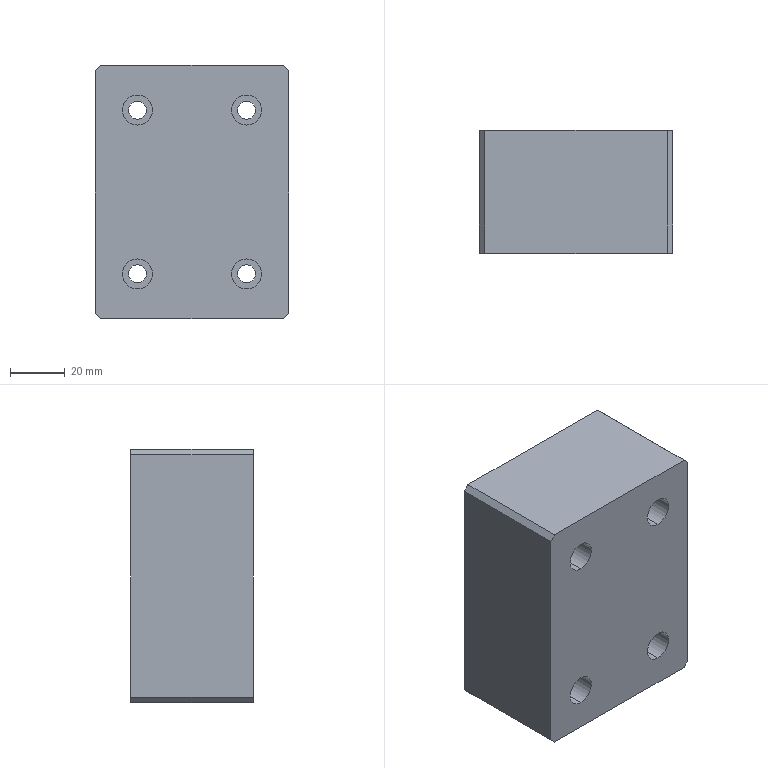Part | STEP file | 11-FG-SJ00911 | 1 solid | 30 faces | box 71 x 45 x 93 mm | volume 285751 mm3 | cylinder 16 | plane 14 | commonest cylinder face diameters 6.6 x8 11 x8
STEP:
#1=CARTESIAN_POINT('',(20.,20.,35.5));
#2=VERTEX_POINT('',#1);
#3=CARTESIAN_POINT('',(20.,20.,24.5));
#4=VERTEX_POINT('',#3);
#5=CARTESIAN_POINT('',(20.,20.,30.));
#6=DIRECTION('',(0.,-1.,0.));
#7=DIRECTION('',(0.,0.,-1.));
#8=AXIS2_PLACEMENT_3D('',#5,#6,#7);
#9=CIRCLE('',#8,5.5);
#10=EDGE_CURVE('',#2,#4,#9,.T.);
#11=ORIENTED_EDGE('',*,*,#10,.F.);
#12=CARTESIAN_POINT('',(20.,0.,35.5));
#13=VERTEX_POINT('',#12);
#14=CARTESIAN_POINT('',(20.,0.,35.5));
#15=DIRECTION('',(0.,-1.,0.));
#16=VECTOR('',#15,1000.);
#17=LINE('',#14,#16);
#18=EDGE_CURVE('',#2,#13,#17,.T.);
#19=ORIENTED_EDGE('',*,*,#18,.T.);
#20=CARTESIAN_POINT('',(20.,0.,24.5));
#21=VERTEX_POINT('',#20);
#22=CARTESIAN_POINT('',(20.,0.,30.));
#23=DIRECTION('',(0.,-1.,0.));
#24=DIRECTION('',(0.,0.,-1.));
#25=AXIS2_PLACEMENT_3D('',#22,#23,#24);
#26=CIRCLE('',#25,5.5);
#27=EDGE_CURVE('',#13,#21,#26,.T.);
#28=ORIENTED_EDGE('',*,*,#27,.T.);
#29=CARTESIAN_POINT('',(20.,0.,24.5));
#30=DIRECTION('',(0.,-1.,0.));
#31=VECTOR('',#30,1000.);
#32=LINE('',#29,#31);
#33=EDGE_CURVE('',#4,#21,#32,.T.);
#34=ORIENTED_EDGE('',*,*,#33,.F.);
#35=EDGE_LOOP('',(#11,#19,#28,#34));
#36=FACE_OUTER_BOUND('',#35,.T.);
#37=CARTESIAN_POINT('',(20.,0.,30.));
#38=DIRECTION('',(0.,-1.,0.));
#39=DIRECTION('',(0.,0.,-1.));
#40=AXIS2_PLACEMENT_3D('',#37,#38,#39);
#41=CYLINDRICAL_SURFACE('',#40,5.5);
#42=ADVANCED_FACE('',(#36),#41,.F.);
#43=CARTESIAN_POINT('',(20.,45.,33.3));
#44=VERTEX_POINT('',#43);
#45=CARTESIAN_POINT('',(20.,45.,26.7));
#46=VERTEX_POINT('',#45);
#47=CARTESIAN_POINT('',(20.,45.,30.));
#48=DIRECTION('',(0.,-1.,0.));
#49=DIRECTION('',(0.,0.,-1.));
#50=AXIS2_PLACEMENT_3D('',#47,#48,#49);
#51=CIRCLE('',#50,3.3);
#52=EDGE_CURVE('',#44,#46,#51,.T.);
#53=ORIENTED_EDGE('',*,*,#52,.F.);
#54=CARTESIAN_POINT('',(20.,20.,33.3));
#55=VERTEX_POINT('',#54);
#56=CARTESIAN_POINT('',(20.,0.,33.3));
#57=DIRECTION('',(0.,-1.,0.));
#58=VECTOR('',#57,1000.);
#59=LINE('',#56,#58);
#60=EDGE_CURVE('',#44,#55,#59,.T.);
#61=ORIENTED_EDGE('',*,*,#60,.T.);
#62=CARTESIAN_POINT('',(20.,20.,26.7));
#63=VERTEX_POINT('',#62);
#64=CARTESIAN_POINT('',(20.,20.,30.));
#65=DIRECTION('',(0.,-1.,0.));
#66=DIRECTION('',(0.,0.,-1.));
#67=AXIS2_PLACEMENT_3D('',#64,#65,#66);
#68=CIRCLE('',#67,3.3);
#69=EDGE_CURVE('',#55,#63,#68,.T.);
#70=ORIENTED_EDGE('',*,*,#69,.T.);
#71=CARTESIAN_POINT('',(20.,0.,26.7));
#72=DIRECTION('',(0.,-1.,0.));
#73=VECTOR('',#72,1000.);
#74=LINE('',#71,#73);
#75=EDGE_CURVE('',#46,#63,#74,.T.);
#76=ORIENTED_EDGE('',*,*,#75,.F.);
#77=EDGE_LOOP('',(#53,#61,#70,#76));
#78=FACE_OUTER_BOUND('',#77,.T.);
#79=CARTESIAN_POINT('',(20.,0.,30.));
#80=DIRECTION('',(0.,-1.,0.));
#81=DIRECTION('',(0.,0.,-1.));
#82=AXIS2_PLACEMENT_3D('',#79,#80,#81);
#83=CYLINDRICAL_SURFACE('',#82,3.3);
#84=ADVANCED_FACE('',(#78),#83,.F.);
#85=CARTESIAN_POINT('',(-20.,20.,35.5));
#86=VERTEX_POINT('',#85);
#87=CARTESIAN_POINT('',(-20.,20.,24.5));
#88=VERTEX_POINT('',#87);
#89=CARTESIAN_POINT('',(-20.,20.,30.));
#90=DIRECTION('',(0.,-1.,0.));
#91=DIRECTION('',(0.,0.,-1.));
#92=AXIS2_PLACEMENT_3D('',#89,#90,#91);
#93=CIRCLE('',#92,5.5);
#94=EDGE_CURVE('',#86,#88,#93,.T.);
#95=ORIENTED_EDGE('',*,*,#94,.F.);
#96=CARTESIAN_POINT('',(-20.,0.,35.5));
#97=VERTEX_POINT('',#96);
#98=CARTESIAN_POINT('',(-20.,0.,35.5));
#99=DIRECTION('',(0.,-1.,0.));
#100=VECTOR('',#99,1000.);
#101=LINE('',#98,#100);
#102=EDGE_CURVE('',#86,#97,#101,.T.);
#103=ORIENTED_EDGE('',*,*,#102,.T.);
#104=CARTESIAN_POINT('',(-20.,0.,24.5));
#105=VERTEX_POINT('',#104);
#106=CARTESIAN_POINT('',(-20.,0.,30.));
#107=DIRECTION('',(0.,-1.,0.));
#108=DIRECTION('',(0.,0.,-1.));
#109=AXIS2_PLACEMENT_3D('',#106,#107,#108);
#110=CIRCLE('',#109,5.5);
#111=EDGE_CURVE('',#97,#105,#110,.T.);
#112=ORIENTED_EDGE('',*,*,#111,.T.);
#113=CARTESIAN_POINT('',(-20.,0.,24.5));
#114=DIRECTION('',(0.,-1.,0.));
#115=VECTOR('',#114,1000.);
#116=LINE('',#113,#115);
#117=EDGE_CURVE('',#88,#105,#116,.T.);
#118=ORIENTED_EDGE('',*,*,#117,.F.);
#119=EDGE_LOOP('',(#95,#103,#112,#118));
#120=FACE_OUTER_BOUND('',#119,.T.);
#121=CARTESIAN_POINT('',(-20.,0.,30.));
#122=DIRECTION('',(0.,-1.,0.));
#123=DIRECTION('',(0.,0.,-1.));
#124=AXIS2_PLACEMENT_3D('',#121,#122,#123);
#125=CYLINDRICAL_SURFACE('',#124,5.5);
#126=ADVANCED_FACE('',(#120),#125,.F.);
#127=CARTESIAN_POINT('',(-20.,45.,33.3));
#128=VERTEX_POINT('',#127);
#129=CARTESIAN_POINT('',(-20.,45.,26.7));
#130=VERTEX_POINT('',#129);
#131=CARTESIAN_POINT('',(-20.,45.,30.));
#132=DIRECTION('',(0.,-1.,0.));
#133=DIRECTION('',(0.,0.,-1.));
#134=AXIS2_PLACEMENT_3D('',#131,#132,#133);
#135=CIRCLE('',#134,3.3);
#136=EDGE_CURVE('',#128,#130,#135,.T.);
#137=ORIENTED_EDGE('',*,*,#136,.F.);
#138=CARTESIAN_POINT('',(-20.,20.,33.3));
#139=VERTEX_POINT('',#138);
#140=CARTESIAN_POINT('',(-20.,0.,33.3));
#141=DIRECTION('',(0.,-1.,0.));
#142=VECTOR('',#141,1000.);
#143=LINE('',#140,#142);
#144=EDGE_CURVE('',#128,#139,#143,.T.);
#145=ORIENTED_EDGE('',*,*,#144,.T.);
#146=CARTESIAN_POINT('',(-20.,20.,26.7));
#147=VERTEX_POINT('',#146);
#148=CARTESIAN_POINT('',(-20.,20.,30.));
#149=DIRECTION('',(0.,-1.,0.));
#150=DIRECTION('',(0.,0.,-1.));
#151=AXIS2_PLACEMENT_3D('',#148,#149,#150);
#152=CIRCLE('',#151,3.3);
#153=EDGE_CURVE('',#139,#147,#152,.T.);
#154=ORIENTED_EDGE('',*,*,#153,.T.);
#155=CARTESIAN_POINT('',(-20.,0.,26.7));
#156=DIRECTION('',(0.,-1.,0.));
#157=VECTOR('',#156,1000.);
#158=LINE('',#155,#157);
#159=EDGE_CURVE('',#130,#147,#158,.T.);
#160=ORIENTED_EDGE('',*,*,#159,.F.);
#161=EDGE_LOOP('',(#137,#145,#154,#160));
#162=FACE_OUTER_BOUND('',#161,.T.);
#163=CARTESIAN_POINT('',(-20.,0.,30.));
#164=DIRECTION('',(0.,-1.,0.));
#165=DIRECTION('',(0.,0.,-1.));
#166=AXIS2_PLACEMENT_3D('',#163,#164,#165);
#167=CYLINDRICAL_SURFACE('',#166,3.3);
#168=ADVANCED_FACE('',(#162),#167,.F.);
#169=CARTESIAN_POINT('',(-20.,20.,-24.5));
#170=VERTEX_POINT('',#169);
#171=CARTESIAN_POINT('',(-20.,20.,-35.5));
#172=VERTEX_POINT('',#171);
#173=CARTESIAN_POINT('',(-20.,20.,-30.));
#174=DIRECTION('',(0.,-1.,0.));
#175=DIRECTION('',(0.,0.,-1.));
#176=AXIS2_PLACEMENT_3D('',#173,#174,#175);
#177=CIRCLE('',#176,5.5);
#178=EDGE_CURVE('',#170,#172,#177,.T.);
#179=ORIENTED_EDGE('',*,*,#178,.F.);
#180=CARTESIAN_POINT('',(-20.,0.,-24.5));
#181=VERTEX_POINT('',#180);
#182=CARTESIAN_POINT('',(-20.,0.,-24.5));
#183=DIRECTION('',(0.,-1.,0.));
#184=VECTOR('',#183,1000.);
#185=LINE('',#182,#184);
#186=EDGE_CURVE('',#170,#181,#185,.T.);
#187=ORIENTED_EDGE('',*,*,#186,.T.);
#188=CARTESIAN_POINT('',(-20.,0.,-35.5));
#189=VERTEX_POINT('',#188);
#190=CARTESIAN_POINT('',(-20.,0.,-30.));
#191=DIRECTION('',(0.,-1.,0.));
#192=DIRECTION('',(0.,0.,-1.));
#193=AXIS2_PLACEMENT_3D('',#190,#191,#192);
#194=CIRCLE('',#193,5.5);
#195=EDGE_CURVE('',#181,#189,#194,.T.);
#196=ORIENTED_EDGE('',*,*,#195,.T.);
#197=CARTESIAN_POINT('',(-20.,0.,-35.5));
#198=DIRECTION('',(0.,-1.,0.));
#199=VECTOR('',#198,1000.);
#200=LINE('',#197,#199);
#201=EDGE_CURVE('',#172,#189,#200,.T.);
#202=ORIENTED_EDGE('',*,*,#201,.F.);
#203=EDGE_LOOP('',(#179,#187,#196,#202));
#204=FACE_OUTER_BOUND('',#203,.T.);
#205=CARTESIAN_POINT('',(-20.,0.,-30.));
#206=DIRECTION('',(0.,-1.,0.));
#207=DIRECTION('',(0.,0.,-1.));
#208=AXIS2_PLACEMENT_3D('',#205,#206,#207);
#209=CYLINDRICAL_SURFACE('',#208,5.5);
#210=ADVANCED_FACE('',(#204),#209,.F.);
#211=CARTESIAN_POINT('',(-20.,45.,-26.7));
#212=VERTEX_POINT('',#211);
#213=CARTESIAN_POINT('',(-20.,45.,-33.3));
#214=VERTEX_POINT('',#213);
#215=CARTESIAN_POINT('',(-20.,45.,-30.));
#216=DIRECTION('',(0.,-1.,0.));
#217=DIRECTION('',(0.,0.,-1.));
#218=AXIS2_PLACEMENT_3D('',#215,#216,#217);
#219=CIRCLE('',#218,3.3);
#220=EDGE_CURVE('',#212,#214,#219,.T.);
#221=ORIENTED_EDGE('',*,*,#220,.F.);
#222=CARTESIAN_POINT('',(-20.,20.,-26.7));
#223=VERTEX_POINT('',#222);
#224=CARTESIAN_POINT('',(-20.,0.,-26.7));
#225=DIRECTION('',(0.,-1.,0.));
#226=VECTOR('',#225,1000.);
#227=LINE('',#224,#226);
#228=EDGE_CURVE('',#212,#223,#227,.T.);
#229=ORIENTED_EDGE('',*,*,#228,.T.);
#230=CARTESIAN_POINT('',(-20.,20.,-33.3));
#231=VERTEX_POINT('',#230);
#232=CARTESIAN_POINT('',(-20.,20.,-30.));
#233=DIRECTION('',(0.,-1.,0.));
#234=DIRECTION('',(0.,0.,-1.));
#235=AXIS2_PLACEMENT_3D('',#232,#233,#234);
#236=CIRCLE('',#235,3.3);
#237=EDGE_CURVE('',#223,#231,#236,.T.);
#238=ORIENTED_EDGE('',*,*,#237,.T.);
#239=CARTESIAN_POINT('',(-20.,0.,-33.3));
#240=DIRECTION('',(0.,-1.,0.));
#241=VECTOR('',#240,1000.);
#242=LINE('',#239,#241);
#243=EDGE_CURVE('',#214,#231,#242,.T.);
#244=ORIENTED_EDGE('',*,*,#243,.F.);
#245=EDGE_LOOP('',(#221,#229,#238,#244));
#246=FACE_OUTER_BOUND('',#245,.T.);
#247=CARTESIAN_POINT('',(-20.,0.,-30.));
#248=DIRECTION('',(0.,-1.,0.));
#249=DIRECTION('',(0.,0.,-1.));
#250=AXIS2_PLACEMENT_3D('',#247,#248,#249);
#251=CYLINDRICAL_SURFACE('',#250,3.3);
#252=ADVANCED_FACE('',(#246),#251,.F.);
#253=CARTESIAN_POINT('',(20.,20.,-24.5));
#254=VERTEX_POINT('',#253);
#255=CARTESIAN_POINT('',(20.,20.,-35.5));
#256=VERTEX_POINT('',#255);
#257=CARTESIAN_POINT('',(20.,20.,-30.));
#258=DIRECTION('',(0.,-1.,0.));
#259=DIRECTION('',(0.,0.,-1.));
#260=AXIS2_PLACEMENT_3D('',#257,#258,#259);
#261=CIRCLE('',#260,5.5);
#262=EDGE_CURVE('',#254,#256,#261,.T.);
#263=ORIENTED_EDGE('',*,*,#262,.F.);
#264=CARTESIAN_POINT('',(20.,0.,-24.5));
#265=VERTEX_POINT('',#264);
#266=CARTESIAN_POINT('',(20.,0.,-24.5));
#267=DIRECTION('',(0.,-1.,0.));
#268=VECTOR('',#267,1000.);
#269=LINE('',#266,#268);
#270=EDGE_CURVE('',#254,#265,#269,.T.);
#271=ORIENTED_EDGE('',*,*,#270,.T.);
#272=CARTESIAN_POINT('',(20.,0.,-35.5));
#273=VERTEX_POINT('',#272);
#274=CARTESIAN_POINT('',(20.,0.,-30.));
#275=DIRECTION('',(0.,-1.,0.));
#276=DIRECTION('',(0.,0.,-1.));
#277=AXIS2_PLACEMENT_3D('',#274,#275,#276);
#278=CIRCLE('',#277,5.5);
#279=EDGE_CURVE('',#265,#273,#278,.T.);
#280=ORIENTED_EDGE('',*,*,#279,.T.);
#281=CARTESIAN_POINT('',(20.,0.,-35.5));
#282=DIRECTION('',(0.,-1.,0.));
#283=VECTOR('',#282,1000.);
#284=LINE('',#281,#283);
#285=EDGE_CURVE('',#256,#273,#284,.T.);
#286=ORIENTED_EDGE('',*,*,#285,.F.);
#287=EDGE_LOOP('',(#263,#271,#280,#286));
#288=FACE_OUTER_BOUND('',#287,.T.);
#289=CARTESIAN_POINT('',(20.,0.,-30.));
#290=DIRECTION('',(0.,-1.,0.));
#291=DIRECTION('',(0.,0.,-1.));
#292=AXIS2_PLACEMENT_3D('',#289,#290,#291);
#293=CYLINDRICAL_SURFACE('',#292,5.5);
#294=ADVANCED_FACE('',(#288),#293,.F.);
#295=CARTESIAN_POINT('',(20.,45.,-26.7));
#296=VERTEX_POINT('',#295);
#297=CARTESIAN_POINT('',(20.,45.,-33.3));
#298=VERTEX_POINT('',#297);
#299=CARTESIAN_POINT('',(20.,45.,-30.));
#300=DIRECTION('',(0.,-1.,0.));
#301=DIRECTION('',(0.,0.,-1.));
#302=AXIS2_PLACEMENT_3D('',#299,#300,#301);
#303=CIRCLE('',#302,3.3);
#304=EDGE_CURVE('',#296,#298,#303,.T.);
#305=ORIENTED_EDGE('',*,*,#304,.F.);
#306=CARTESIAN_POINT('',(20.,20.,-26.7));
#307=VERTEX_POINT('',#306);
#308=CARTESIAN_POINT('',(20.,0.,-26.7));
#309=DIRECTION('',(0.,-1.,0.));
#310=VECTOR('',#309,1000.);
#311=LINE('',#308,#310);
#312=EDGE_CURVE('',#296,#307,#311,.T.);
#313=ORIENTED_EDGE('',*,*,#312,.T.);
#314=CARTESIAN_POINT('',(20.,20.,-33.3));
#315=VERTEX_POINT('',#314);
#316=CARTESIAN_POINT('',(20.,20.,-30.));
#317=DIRECTION('',(0.,-1.,0.));
#318=DIRECTION('',(0.,0.,-1.));
#319=AXIS2_PLACEMENT_3D('',#316,#317,#318);
#320=CIRCLE('',#319,3.3);
#321=EDGE_CURVE('',#307,#315,#320,.T.);
#322=ORIENTED_EDGE('',*,*,#321,.T.);
#323=CARTESIAN_POINT('',(20.,0.,-33.3));
#324=DIRECTION('',(0.,-1.,0.));
#325=VECTOR('',#324,1000.);
#326=LINE('',#323,#325);
#327=EDGE_CURVE('',#298,#315,#326,.T.);
#328=ORIENTED_EDGE('',*,*,#327,.F.);
#329=EDGE_LOOP('',(#305,#313,#322,#328));
#330=FACE_OUTER_BOUND('',#329,.T.);
#331=CARTESIAN_POINT('',(20.,0.,-30.));
#332=DIRECTION('',(0.,-1.,0.));
#333=DIRECTION('',(0.,0.,-1.));
#334=AXIS2_PLACEMENT_3D('',#331,#332,#333);
#335=CYLINDRICAL_SURFACE('',#334,3.3);
#336=ADVANCED_FACE('',(#330),#335,.F.);
#337=CARTESIAN_POINT('',(-35.5,0.,-44.5));
#338=VERTEX_POINT('',#337);
#339=CARTESIAN_POINT('',(-35.5,0.,44.5));
#340=VERTEX_POINT('',#339);
#341=CARTESIAN_POINT('',(-35.5,0.,46.5));
#342=DIRECTION('',(0.,0.,1.));
#343=VECTOR('',#342,1000.);
#344=LINE('',#341,#343);
#345=EDGE_CURVE('',#338,#340,#344,.T.);
#346=ORIENTED_EDGE('',*,*,#345,.T.);
#347=CARTESIAN_POINT('',(-35.5,45.,44.5));
#348=VERTEX_POINT('',#347);
#349=CARTESIAN_POINT('',(-35.5,45.,44.5));
#350=DIRECTION('',(0.,1.,0.));
#351=VECTOR('',#350,1000.);
#352=LINE('',#349,#351);
#353=EDGE_CURVE('',#340,#348,#352,.T.);
#354=ORIENTED_EDGE('',*,*,#353,.T.);
#355=CARTESIAN_POINT('',(-35.5,45.,-44.5));
#356=VERTEX_POINT('',#355);
#357=CARTESIAN_POINT('',(-35.5,45.,46.5));
#358=DIRECTION('',(0.,0.,1.));
#359=VECTOR('',#358,1000.);
#360=LINE('',#357,#359);
#361=EDGE_CURVE('',#356,#348,#360,.T.);
#362=ORIENTED_EDGE('',*,*,#361,.F.);
#363=CARTESIAN_POINT('',(-35.5,45.,-44.5));
#364=DIRECTION('',(0.,-1.,0.));
#365=VECTOR('',#364,1000.);
#366=LINE('',#363,#365);
#367=EDGE_CURVE('',#356,#338,#366,.T.);
#368=ORIENTED_EDGE('',*,*,#367,.T.);
#369=EDGE_LOOP('',(#346,#354,#362,#368));
#370=FACE_OUTER_BOUND('',#369,.T.);
#371=CARTESIAN_POINT('',(-35.5,45.,46.5));
#372=DIRECTION('',(1.,0.,0.));
#373=DIRECTION('',(0.,0.,-1.));
#374=AXIS2_PLACEMENT_3D('',#371,#372,#373);
#375=PLANE('',#374);
#376=ADVANCED_FACE('',(#370),#375,.F.);
#377=CARTESIAN_POINT('',(-33.5,45.,46.5));
#378=VERTEX_POINT('',#377);
#379=CARTESIAN_POINT('',(33.5,45.,46.5));
#380=VERTEX_POINT('',#379);
#381=CARTESIAN_POINT('',(35.5,45.,46.5));
#382=DIRECTION('',(1.,0.,0.));
#383=VECTOR('',#382,1000.);
#384=LINE('',#381,#383);
#385=EDGE_CURVE('',#378,#380,#384,.T.);
#386=ORIENTED_EDGE('',*,*,#385,.F.);
#387=CARTESIAN_POINT('',(-33.5,0.,46.5));
#388=VERTEX_POINT('',#387);
#389=CARTESIAN_POINT('',(-33.5,45.,46.5));
#390=DIRECTION('',(0.,-1.,0.));
#391=VECTOR('',#390,1000.);
#392=LINE('',#389,#391);
#393=EDGE_CURVE('',#378,#388,#392,.T.);
#394=ORIENTED_EDGE('',*,*,#393,.T.);
#395=CARTESIAN_POINT('',(33.5,0.,46.5));
#396=VERTEX_POINT('',#395);
#397=CARTESIAN_POINT('',(35.5,0.,46.5));
#398=DIRECTION('',(1.,0.,0.));
#399=VECTOR('',#398,1000.);
#400=LINE('',#397,#399);
#401=EDGE_CURVE('',#388,#396,#400,.T.);
#402=ORIENTED_EDGE('',*,*,#401,.T.);
#403=CARTESIAN_POINT('',(33.5,45.,46.5));
#404=DIRECTION('',(0.,1.,0.));
#405=VECTOR('',#404,1000.);
#406=LINE('',#403,#405);
#407=EDGE_CURVE('',#396,#380,#406,.T.);
#408=ORIENTED_EDGE('',*,*,#407,.T.);
#409=EDGE_LOOP('',(#386,#394,#402,#408));
#410=FACE_OUTER_BOUND('',#409,.T.);
#411=CARTESIAN_POINT('',(35.5,45.,46.5));
#412=DIRECTION('',(0.,0.,-1.));
#413=DIRECTION('',(-1.,0.,0.));
#414=AXIS2_PLACEMENT_3D('',#411,#412,#413);
#415=PLANE('',#414);
#416=ADVANCED_FACE('',(#410),#415,.F.);
#417=CARTESIAN_POINT('',(35.5,45.,44.5));
#418=VERTEX_POINT('',#417);
#419=CARTESIAN_POINT('',(35.5,45.,-44.5));
#420=VERTEX_POINT('',#419);
#421=CARTESIAN_POINT('',(35.5,45.,46.5));
#422=DIRECTION('',(0.,0.,-1.));
#423=VECTOR('',#422,1000.);
#424=LINE('',#421,#423);
#425=EDGE_CURVE('',#418,#420,#424,.T.);
#426=ORIENTED_EDGE('',*,*,#425,.F.);
#427=CARTESIAN_POINT('',(35.5,0.,44.5));
#428=VERTEX_POINT('',#427);
#429=CARTESIAN_POINT('',(35.5,45.,44.5));
#430=DIRECTION('',(0.,-1.,0.));
#431=VECTOR('',#430,1000.);
#432=LINE('',#429,#431);
#433=EDGE_CURVE('',#418,#428,#432,.T.);
#434=ORIENTED_EDGE('',*,*,#433,.T.);
#435=CARTESIAN_POINT('',(35.5,0.,-44.5));
#436=VERTEX_POINT('',#435);
#437=CARTESIAN_POINT('',(35.5,0.,46.5));
#438=DIRECTION('',(0.,0.,-1.));
#439=VECTOR('',#438,1000.);
#440=LINE('',#437,#439);
#441=EDGE_CURVE('',#428,#436,#440,.T.);
#442=ORIENTED_EDGE('',*,*,#441,.T.);
#443=CARTESIAN_POINT('',(35.5,45.,-44.5));
#444=DIRECTION('',(0.,1.,0.));
#445=VECTOR('',#444,1000.);
#446=LINE('',#443,#445);
#447=EDGE_CURVE('',#436,#420,#446,.T.);
#448=ORIENTED_EDGE('',*,*,#447,.T.);
#449=EDGE_LOOP('',(#426,#434,#442,#448));
#450=FACE_OUTER_BOUND('',#449,.T.);
#451=CARTESIAN_POINT('',(35.5,45.,46.5));
#452=DIRECTION('',(-1.,0.,0.));
#453=DIRECTION('',(0.,0.,1.));
#454=AXIS2_PLACEMENT_3D('',#451,#452,#453);
#455=PLANE('',#454);
#456=ADVANCED_FACE('',(#450),#455,.F.);
#457=CARTESIAN_POINT('',(33.5,0.,-46.5));
#458=VERTEX_POINT('',#457);
#459=CARTESIAN_POINT('',(-33.5,0.,-46.5));
#460=VERTEX_POINT('',#459);
#461=CARTESIAN_POINT('',(35.5,0.,-46.5));
#462=DIRECTION('',(-1.,0.,0.));
#463=VECTOR('',#462,1000.);
#464=LINE('',#461,#463);
#465=EDGE_CURVE('',#458,#460,#464,.T.);
#466=ORIENTED_EDGE('',*,*,#465,.T.);
#467=CARTESIAN_POINT('',(-33.5,45.,-46.5));
#468=VERTEX_POINT('',#467);
#469=CARTESIAN_POINT('',(-33.5,45.,-46.5));
#470=DIRECTION('',(0.,1.,0.));
#471=VECTOR('',#470,1000.);
#472=LINE('',#469,#471);
#473=EDGE_CURVE('',#460,#468,#472,.T.);
#474=ORIENTED_EDGE('',*,*,#473,.T.);
#475=CARTESIAN_POINT('',(33.5,45.,-46.5));
#476=VERTEX_POINT('',#475);
#477=CARTESIAN_POINT('',(35.5,45.,-46.5));
#478=DIRECTION('',(-1.,0.,0.));
#479=VECTOR('',#478,1000.);
#480=LINE('',#477,#479);
#481=EDGE_CURVE('',#476,#468,#480,.T.);
#482=ORIENTED_EDGE('',*,*,#481,.F.);
#483=CARTESIAN_POINT('',(33.5,45.,-46.5));
#484=DIRECTION('',(0.,-1.,0.));
#485=VECTOR('',#484,1000.);
#486=LINE('',#483,#485);
#487=EDGE_CURVE('',#476,#458,#486,.T.);
#488=ORIENTED_EDGE('',*,*,#487,.T.);
#489=EDGE_LOOP('',(#466,#474,#482,#488));
#490=FACE_OUTER_BOUND('',#489,.T.);
#491=CARTESIAN_POINT('',(35.5,45.,-46.5));
#492=DIRECTION('',(0.,0.,1.));
#493=DIRECTION('',(1.,0.,0.));
#494=AXIS2_PLACEMENT_3D('',#491,#492,#493);
#495=PLANE('',#494);
#496=ADVANCED_FACE('',(#490),#495,.F.);
#497=CARTESIAN_POINT('',(20.,45.,30.));
#498=DIRECTION('',(0.,-1.,0.));
#499=DIRECTION('',(0.,0.,-1.));
#500=AXIS2_PLACEMENT_3D('',#497,#498,#499);
#501=CIRCLE('',#500,3.3);
#502=EDGE_CURVE('',#46,#44,#501,.T.);
#503=ORIENTED_EDGE('',*,*,#502,.T.);
#504=ORIENTED_EDGE('',*,*,#52,.T.);
#505=EDGE_LOOP('',(#503,#504));
#506=FACE_BOUND('',#505,.T.);
#507=CARTESIAN_POINT('',(-20.,45.,30.));
#508=DIRECTION('',(0.,-1.,0.));
#509=DIRECTION('',(0.,0.,-1.));
#510=AXIS2_PLACEMENT_3D('',#507,#508,#509);
#511=CIRCLE('',#510,3.3);
#512=EDGE_CURVE('',#130,#128,#511,.T.);
#513=ORIENTED_EDGE('',*,*,#512,.T.);
#514=ORIENTED_EDGE('',*,*,#136,.T.);
#515=EDGE_LOOP('',(#513,#514));
#516=FACE_BOUND('',#515,.T.);
#517=CARTESIAN_POINT('',(-20.,45.,-30.));
#518=DIRECTION('',(0.,-1.,0.));
#519=DIRECTION('',(0.,0.,-1.));
#520=AXIS2_PLACEMENT_3D('',#517,#518,#519);
#521=CIRCLE('',#520,3.3);
#522=EDGE_CURVE('',#214,#212,#521,.T.);
#523=ORIENTED_EDGE('',*,*,#522,.T.);
#524=ORIENTED_EDGE('',*,*,#220,.T.);
#525=EDGE_LOOP('',(#523,#524));
#526=FACE_BOUND('',#525,.T.);
#527=CARTESIAN_POINT('',(20.,45.,-30.));
#528=DIRECTION('',(0.,-1.,0.));
#529=DIRECTION('',(0.,0.,-1.));
#530=AXIS2_PLACEMENT_3D('',#527,#528,#529);
#531=CIRCLE('',#530,3.3);
#532=EDGE_CURVE('',#298,#296,#531,.T.);
#533=ORIENTED_EDGE('',*,*,#532,.T.);
#534=ORIENTED_EDGE('',*,*,#304,.T.);
#535=EDGE_LOOP('',(#533,#534));
#536=FACE_BOUND('',#535,.T.);
#537=ORIENTED_EDGE('',*,*,#361,.T.);
#538=CARTESIAN_POINT('',(-40.,45.,40.));
#539=DIRECTION('',(0.7071,0.,0.7071));
#540=VECTOR('',#539,1000.);
#541=LINE('',#538,#540);
#542=EDGE_CURVE('',#348,#378,#541,.T.);
#543=ORIENTED_EDGE('',*,*,#542,.T.);
#544=ORIENTED_EDGE('',*,*,#385,.T.);
#545=CARTESIAN_POINT('',(40.,45.,40.));
#546=DIRECTION('',(0.7071,0.,-0.7071));
#547=VECTOR('',#546,1000.);
#548=LINE('',#545,#547);
#549=EDGE_CURVE('',#380,#418,#548,.T.);
#550=ORIENTED_EDGE('',*,*,#549,.T.);
#551=ORIENTED_EDGE('',*,*,#425,.T.);
#552=CARTESIAN_POINT('',(40.,45.,-40.));
#553=DIRECTION('',(-0.7071,0.,-0.7071));
#554=VECTOR('',#553,1000.);
#555=LINE('',#552,#554);
#556=EDGE_CURVE('',#420,#476,#555,.T.);
#557=ORIENTED_EDGE('',*,*,#556,.T.);
#558=ORIENTED_EDGE('',*,*,#481,.T.);
#559=CARTESIAN_POINT('',(-40.,45.,-40.));
#560=DIRECTION('',(-0.7071,0.,0.7071));
#561=VECTOR('',#560,1000.);
#562=LINE('',#559,#561);
#563=EDGE_CURVE('',#468,#356,#562,.T.);
#564=ORIENTED_EDGE('',*,*,#563,.T.);
#565=EDGE_LOOP('',(#537,#543,#544,#550,#551,#557,#558,#564));
#566=FACE_OUTER_BOUND('',#565,.T.);
#567=CARTESIAN_POINT('',(0.,45.,0.));
#568=DIRECTION('',(0.,1.,0.));
#569=DIRECTION('',(0.,0.,1.));
#570=AXIS2_PLACEMENT_3D('',#567,#568,#569);
#571=PLANE('',#570);
#572=ADVANCED_FACE('',(#506,#516,#526,#536,#566),#571,.T.);
#573=CARTESIAN_POINT('',(20.,0.,30.));
#574=DIRECTION('',(0.,-1.,0.));
#575=DIRECTION('',(0.,0.,-1.));
#576=AXIS2_PLACEMENT_3D('',#573,#574,#575);
#577=CIRCLE('',#576,5.5);
#578=EDGE_CURVE('',#21,#13,#577,.T.);
#579=ORIENTED_EDGE('',*,*,#578,.F.);
#580=ORIENTED_EDGE('',*,*,#27,.F.);
#581=EDGE_LOOP('',(#579,#580));
#582=FACE_BOUND('',#581,.T.);
#583=CARTESIAN_POINT('',(-20.,0.,30.));
#584=DIRECTION('',(0.,-1.,0.));
#585=DIRECTION('',(0.,0.,-1.));
#586=AXIS2_PLACEMENT_3D('',#583,#584,#585);
#587=CIRCLE('',#586,5.5);
#588=EDGE_CURVE('',#105,#97,#587,.T.);
#589=ORIENTED_EDGE('',*,*,#588,.F.);
#590=ORIENTED_EDGE('',*,*,#111,.F.);
#591=EDGE_LOOP('',(#589,#590));
#592=FACE_BOUND('',#591,.T.);
#593=CARTESIAN_POINT('',(-20.,0.,-30.));
#594=DIRECTION('',(0.,-1.,0.));
#595=DIRECTION('',(0.,0.,-1.));
#596=AXIS2_PLACEMENT_3D('',#593,#594,#595);
#597=CIRCLE('',#596,5.5);
#598=EDGE_CURVE('',#189,#181,#597,.T.);
#599=ORIENTED_EDGE('',*,*,#598,.F.);
#600=ORIENTED_EDGE('',*,*,#195,.F.);
#601=EDGE_LOOP('',(#599,#600));
#602=FACE_BOUND('',#601,.T.);
#603=CARTESIAN_POINT('',(20.,0.,-30.));
#604=DIRECTION('',(0.,-1.,0.));
#605=DIRECTION('',(0.,0.,-1.));
#606=AXIS2_PLACEMENT_3D('',#603,#604,#605);
#607=CIRCLE('',#606,5.5);
#608=EDGE_CURVE('',#273,#265,#607,.T.);
#609=ORIENTED_EDGE('',*,*,#608,.F.);
#610=ORIENTED_EDGE('',*,*,#279,.F.);
#611=EDGE_LOOP('',(#609,#610));
#612=FACE_BOUND('',#611,.T.);
#613=ORIENTED_EDGE('',*,*,#401,.F.);
#614=CARTESIAN_POINT('',(-33.5,0.,46.5));
#615=DIRECTION('',(-0.7071,0.,-0.7071));
#616=VECTOR('',#615,1000.);
#617=LINE('',#614,#616);
#618=EDGE_CURVE('',#388,#340,#617,.T.);
#619=ORIENTED_EDGE('',*,*,#618,.T.);
#620=ORIENTED_EDGE('',*,*,#345,.F.);
#621=CARTESIAN_POINT('',(-35.5,0.,-44.5));
#622=DIRECTION('',(0.7071,0.,-0.7071));
#623=VECTOR('',#622,1000.);
#624=LINE('',#621,#623);
#625=EDGE_CURVE('',#338,#460,#624,.T.);
#626=ORIENTED_EDGE('',*,*,#625,.T.);
#627=ORIENTED_EDGE('',*,*,#465,.F.);
#628=CARTESIAN_POINT('',(33.5,0.,-46.5));
#629=DIRECTION('',(0.7071,0.,0.7071));
#630=VECTOR('',#629,1000.);
#631=LINE('',#628,#630);
#632=EDGE_CURVE('',#458,#436,#631,.T.);
#633=ORIENTED_EDGE('',*,*,#632,.T.);
#634=ORIENTED_EDGE('',*,*,#441,.F.);
#635=CARTESIAN_POINT('',(35.5,0.,44.5));
#636=DIRECTION('',(-0.7071,0.,0.7071));
#637=VECTOR('',#636,1000.);
#638=LINE('',#635,#637);
#639=EDGE_CURVE('',#428,#396,#638,.T.);
#640=ORIENTED_EDGE('',*,*,#639,.T.);
#641=EDGE_LOOP('',(#613,#619,#620,#626,#627,#633,#634,#640));
#642=FACE_OUTER_BOUND('',#641,.T.);
#643=CARTESIAN_POINT('',(0.,0.,0.));
#644=DIRECTION('',(0.,1.,0.));
#645=DIRECTION('',(0.,0.,1.));
#646=AXIS2_PLACEMENT_3D('',#643,#644,#645);
#647=PLANE('',#646);
#648=ADVANCED_FACE('',(#582,#592,#602,#612,#642),#647,.F.);
#649=ORIENTED_EDGE('',*,*,#312,.F.);
#650=ORIENTED_EDGE('',*,*,#532,.F.);
#651=ORIENTED_EDGE('',*,*,#327,.T.);
#652=CARTESIAN_POINT('',(20.,20.,-30.));
#653=DIRECTION('',(0.,-1.,0.));
#654=DIRECTION('',(0.,0.,-1.));
#655=AXIS2_PLACEMENT_3D('',#652,#653,#654);
#656=CIRCLE('',#655,3.3);
#657=EDGE_CURVE('',#315,#307,#656,.T.);
#658=ORIENTED_EDGE('',*,*,#657,.T.);
#659=EDGE_LOOP('',(#649,#650,#651,#658));
#660=FACE_OUTER_BOUND('',#659,.T.);
#661=CARTESIAN_POINT('',(20.,0.,-30.));
#662=DIRECTION('',(0.,-1.,0.));
#663=DIRECTION('',(0.,0.,-1.));
#664=AXIS2_PLACEMENT_3D('',#661,#662,#663);
#665=CYLINDRICAL_SURFACE('',#664,3.3);
#666=ADVANCED_FACE('',(#660),#665,.F.);
#667=ORIENTED_EDGE('',*,*,#657,.F.);
#668=ORIENTED_EDGE('',*,*,#321,.F.);
#669=EDGE_LOOP('',(#667,#668));
#670=FACE_BOUND('',#669,.T.);
#671=CARTESIAN_POINT('',(20.,20.,-30.));
#672=DIRECTION('',(0.,-1.,0.));
#673=DIRECTION('',(0.,0.,-1.));
#674=AXIS2_PLACEMENT_3D('',#671,#672,#673);
#675=CIRCLE('',#674,5.5);
#676=EDGE_CURVE('',#256,#254,#675,.T.);
#677=ORIENTED_EDGE('',*,*,#676,.T.);
#678=ORIENTED_EDGE('',*,*,#262,.T.);
#679=EDGE_LOOP('',(#677,#678));
#680=FACE_OUTER_BOUND('',#679,.T.);
#681=CARTESIAN_POINT('',(23.3,20.,-30.));
#682=DIRECTION('',(0.,1.,0.));
#683=DIRECTION('',(0.,0.,1.));
#684=AXIS2_PLACEMENT_3D('',#681,#682,#683);
#685=PLANE('',#684);
#686=ADVANCED_FACE('',(#670,#680),#685,.F.);
#687=ORIENTED_EDGE('',*,*,#270,.F.);
#688=ORIENTED_EDGE('',*,*,#676,.F.);
#689=ORIENTED_EDGE('',*,*,#285,.T.);
#690=ORIENTED_EDGE('',*,*,#608,.T.);
#691=EDGE_LOOP('',(#687,#688,#689,#690));
#692=FACE_OUTER_BOUND('',#691,.T.);
#693=CARTESIAN_POINT('',(20.,0.,-30.));
#694=DIRECTION('',(0.,-1.,0.));
#695=DIRECTION('',(0.,0.,-1.));
#696=AXIS2_PLACEMENT_3D('',#693,#694,#695);
#697=CYLINDRICAL_SURFACE('',#696,5.5);
#698=ADVANCED_FACE('',(#692),#697,.F.);
#699=ORIENTED_EDGE('',*,*,#228,.F.);
#700=ORIENTED_EDGE('',*,*,#522,.F.);
#701=ORIENTED_EDGE('',*,*,#243,.T.);
#702=CARTESIAN_POINT('',(-20.,20.,-30.));
#703=DIRECTION('',(0.,-1.,0.));
#704=DIRECTION('',(0.,0.,-1.));
#705=AXIS2_PLACEMENT_3D('',#702,#703,#704);
#706=CIRCLE('',#705,3.3);
#707=EDGE_CURVE('',#231,#223,#706,.T.);
#708=ORIENTED_EDGE('',*,*,#707,.T.);
#709=EDGE_LOOP('',(#699,#700,#701,#708));
#710=FACE_OUTER_BOUND('',#709,.T.);
#711=CARTESIAN_POINT('',(-20.,0.,-30.));
#712=DIRECTION('',(0.,-1.,0.));
#713=DIRECTION('',(0.,0.,-1.));
#714=AXIS2_PLACEMENT_3D('',#711,#712,#713);
#715=CYLINDRICAL_SURFACE('',#714,3.3);
#716=ADVANCED_FACE('',(#710),#715,.F.);
#717=ORIENTED_EDGE('',*,*,#707,.F.);
#718=ORIENTED_EDGE('',*,*,#237,.F.);
#719=EDGE_LOOP('',(#717,#718));
#720=FACE_BOUND('',#719,.T.);
#721=CARTESIAN_POINT('',(-20.,20.,-30.));
#722=DIRECTION('',(0.,-1.,0.));
#723=DIRECTION('',(0.,0.,-1.));
#724=AXIS2_PLACEMENT_3D('',#721,#722,#723);
#725=CIRCLE('',#724,5.5);
#726=EDGE_CURVE('',#172,#170,#725,.T.);
#727=ORIENTED_EDGE('',*,*,#726,.T.);
#728=ORIENTED_EDGE('',*,*,#178,.T.);
#729=EDGE_LOOP('',(#727,#728));
#730=FACE_OUTER_BOUND('',#729,.T.);
#731=CARTESIAN_POINT('',(-16.7,20.,-30.));
#732=DIRECTION('',(0.,1.,0.));
#733=DIRECTION('',(0.,0.,1.));
#734=AXIS2_PLACEMENT_3D('',#731,#732,#733);
#735=PLANE('',#734);
#736=ADVANCED_FACE('',(#720,#730),#735,.F.);
#737=ORIENTED_EDGE('',*,*,#186,.F.);
#738=ORIENTED_EDGE('',*,*,#726,.F.);
#739=ORIENTED_EDGE('',*,*,#201,.T.);
#740=ORIENTED_EDGE('',*,*,#598,.T.);
#741=EDGE_LOOP('',(#737,#738,#739,#740));
#742=FACE_OUTER_BOUND('',#741,.T.);
#743=CARTESIAN_POINT('',(-20.,0.,-30.));
#744=DIRECTION('',(0.,-1.,0.));
#745=DIRECTION('',(0.,0.,-1.));
#746=AXIS2_PLACEMENT_3D('',#743,#744,#745);
#747=CYLINDRICAL_SURFACE('',#746,5.5);
#748=ADVANCED_FACE('',(#742),#747,.F.);
#749=ORIENTED_EDGE('',*,*,#144,.F.);
#750=ORIENTED_EDGE('',*,*,#512,.F.);
#751=ORIENTED_EDGE('',*,*,#159,.T.);
#752=CARTESIAN_POINT('',(-20.,20.,30.));
#753=DIRECTION('',(0.,-1.,0.));
#754=DIRECTION('',(0.,0.,-1.));
#755=AXIS2_PLACEMENT_3D('',#752,#753,#754);
#756=CIRCLE('',#755,3.3);
#757=EDGE_CURVE('',#147,#139,#756,.T.);
#758=ORIENTED_EDGE('',*,*,#757,.T.);
#759=EDGE_LOOP('',(#749,#750,#751,#758));
#760=FACE_OUTER_BOUND('',#759,.T.);
#761=CARTESIAN_POINT('',(-20.,0.,30.));
#762=DIRECTION('',(0.,-1.,0.));
#763=DIRECTION('',(0.,0.,-1.));
#764=AXIS2_PLACEMENT_3D('',#761,#762,#763);
#765=CYLINDRICAL_SURFACE('',#764,3.3);
#766=ADVANCED_FACE('',(#760),#765,.F.);
#767=ORIENTED_EDGE('',*,*,#757,.F.);
#768=ORIENTED_EDGE('',*,*,#153,.F.);
#769=EDGE_LOOP('',(#767,#768));
#770=FACE_BOUND('',#769,.T.);
#771=CARTESIAN_POINT('',(-20.,20.,30.));
#772=DIRECTION('',(0.,-1.,0.));
#773=DIRECTION('',(0.,0.,-1.));
#774=AXIS2_PLACEMENT_3D('',#771,#772,#773);
#775=CIRCLE('',#774,5.5);
#776=EDGE_CURVE('',#88,#86,#775,.T.);
#777=ORIENTED_EDGE('',*,*,#776,.T.);
#778=ORIENTED_EDGE('',*,*,#94,.T.);
#779=EDGE_LOOP('',(#777,#778));
#780=FACE_OUTER_BOUND('',#779,.T.);
#781=CARTESIAN_POINT('',(-16.7,20.,30.));
#782=DIRECTION('',(0.,1.,0.));
#783=DIRECTION('',(0.,0.,1.));
#784=AXIS2_PLACEMENT_3D('',#781,#782,#783);
#785=PLANE('',#784);
#786=ADVANCED_FACE('',(#770,#780),#785,.F.);
#787=ORIENTED_EDGE('',*,*,#102,.F.);
#788=ORIENTED_EDGE('',*,*,#776,.F.);
#789=ORIENTED_EDGE('',*,*,#117,.T.);
#790=ORIENTED_EDGE('',*,*,#588,.T.);
#791=EDGE_LOOP('',(#787,#788,#789,#790));
#792=FACE_OUTER_BOUND('',#791,.T.);
#793=CARTESIAN_POINT('',(-20.,0.,30.));
#794=DIRECTION('',(0.,-1.,0.));
#795=DIRECTION('',(0.,0.,-1.));
#796=AXIS2_PLACEMENT_3D('',#793,#794,#795);
#797=CYLINDRICAL_SURFACE('',#796,5.5);
#798=ADVANCED_FACE('',(#792),#797,.F.);
#799=ORIENTED_EDGE('',*,*,#60,.F.);
#800=ORIENTED_EDGE('',*,*,#502,.F.);
#801=ORIENTED_EDGE('',*,*,#75,.T.);
#802=CARTESIAN_POINT('',(20.,20.,30.));
#803=DIRECTION('',(0.,-1.,0.));
#804=DIRECTION('',(0.,0.,-1.));
#805=AXIS2_PLACEMENT_3D('',#802,#803,#804);
#806=CIRCLE('',#805,3.3);
#807=EDGE_CURVE('',#63,#55,#806,.T.);
#808=ORIENTED_EDGE('',*,*,#807,.T.);
#809=EDGE_LOOP('',(#799,#800,#801,#808));
#810=FACE_OUTER_BOUND('',#809,.T.);
#811=CARTESIAN_POINT('',(20.,0.,30.));
#812=DIRECTION('',(0.,-1.,0.));
#813=DIRECTION('',(0.,0.,-1.));
#814=AXIS2_PLACEMENT_3D('',#811,#812,#813);
#815=CYLINDRICAL_SURFACE('',#814,3.3);
#816=ADVANCED_FACE('',(#810),#815,.F.);
#817=ORIENTED_EDGE('',*,*,#807,.F.);
#818=ORIENTED_EDGE('',*,*,#69,.F.);
#819=EDGE_LOOP('',(#817,#818));
#820=FACE_BOUND('',#819,.T.);
#821=CARTESIAN_POINT('',(20.,20.,30.));
#822=DIRECTION('',(0.,-1.,0.));
#823=DIRECTION('',(0.,0.,-1.));
#824=AXIS2_PLACEMENT_3D('',#821,#822,#823);
#825=CIRCLE('',#824,5.5);
#826=EDGE_CURVE('',#4,#2,#825,.T.);
#827=ORIENTED_EDGE('',*,*,#826,.T.);
#828=ORIENTED_EDGE('',*,*,#10,.T.);
#829=EDGE_LOOP('',(#827,#828));
#830=FACE_OUTER_BOUND('',#829,.T.);
#831=CARTESIAN_POINT('',(23.3,20.,30.));
#832=DIRECTION('',(0.,1.,0.));
#833=DIRECTION('',(0.,0.,1.));
#834=AXIS2_PLACEMENT_3D('',#831,#832,#833);
#835=PLANE('',#834);
#836=ADVANCED_FACE('',(#820,#830),#835,.F.);
#837=ORIENTED_EDGE('',*,*,#18,.F.);
#838=ORIENTED_EDGE('',*,*,#826,.F.);
#839=ORIENTED_EDGE('',*,*,#33,.T.);
#840=ORIENTED_EDGE('',*,*,#578,.T.);
#841=EDGE_LOOP('',(#837,#838,#839,#840));
#842=FACE_OUTER_BOUND('',#841,.T.);
#843=CARTESIAN_POINT('',(20.,0.,30.));
#844=DIRECTION('',(0.,-1.,0.));
#845=DIRECTION('',(0.,0.,-1.));
#846=AXIS2_PLACEMENT_3D('',#843,#844,#845);
#847=CYLINDRICAL_SURFACE('',#846,5.5);
#848=ADVANCED_FACE('',(#842),#847,.F.);
#849=ORIENTED_EDGE('',*,*,#542,.F.);
#850=ORIENTED_EDGE('',*,*,#353,.F.);
#851=ORIENTED_EDGE('',*,*,#618,.F.);
#852=ORIENTED_EDGE('',*,*,#393,.F.);
#853=EDGE_LOOP('',(#849,#850,#851,#852));
#854=FACE_OUTER_BOUND('',#853,.T.);
#855=CARTESIAN_POINT('',(-33.5,45.,46.5));
#856=DIRECTION('',(0.7071,0.,-0.7071));
#857=DIRECTION('',(0.,-1.,0.));
#858=AXIS2_PLACEMENT_3D('',#855,#856,#857);
#859=PLANE('',#858);
#860=ADVANCED_FACE('',(#854),#859,.F.);
#861=ORIENTED_EDGE('',*,*,#549,.F.);
#862=ORIENTED_EDGE('',*,*,#407,.F.);
#863=ORIENTED_EDGE('',*,*,#639,.F.);
#864=ORIENTED_EDGE('',*,*,#433,.F.);
#865=EDGE_LOOP('',(#861,#862,#863,#864));
#866=FACE_OUTER_BOUND('',#865,.T.);
#867=CARTESIAN_POINT('',(35.5,45.,44.5));
#868=DIRECTION('',(-0.7071,0.,-0.7071));
#869=DIRECTION('',(0.,-1.,0.));
#870=AXIS2_PLACEMENT_3D('',#867,#868,#869);
#871=PLANE('',#870);
#872=ADVANCED_FACE('',(#866),#871,.F.);
#873=ORIENTED_EDGE('',*,*,#563,.F.);
#874=ORIENTED_EDGE('',*,*,#473,.F.);
#875=ORIENTED_EDGE('',*,*,#625,.F.);
#876=ORIENTED_EDGE('',*,*,#367,.F.);
#877=EDGE_LOOP('',(#873,#874,#875,#876));
#878=FACE_OUTER_BOUND('',#877,.T.);
#879=CARTESIAN_POINT('',(-35.5,45.,-44.5));
#880=DIRECTION('',(0.7071,0.,0.7071));
#881=DIRECTION('',(0.,-1.,0.));
#882=AXIS2_PLACEMENT_3D('',#879,#880,#881);
#883=PLANE('',#882);
#884=ADVANCED_FACE('',(#878),#883,.F.);
#885=ORIENTED_EDGE('',*,*,#556,.F.);
#886=ORIENTED_EDGE('',*,*,#447,.F.);
#887=ORIENTED_EDGE('',*,*,#632,.F.);
#888=ORIENTED_EDGE('',*,*,#487,.F.);
#889=EDGE_LOOP('',(#885,#886,#887,#888));
#890=FACE_OUTER_BOUND('',#889,.T.);
#891=CARTESIAN_POINT('',(33.5,45.,-46.5));
#892=DIRECTION('',(-0.7071,0.,0.7071));
#893=DIRECTION('',(0.,-1.,0.));
#894=AXIS2_PLACEMENT_3D('',#891,#892,#893);
#895=PLANE('',#894);
#896=ADVANCED_FACE('',(#890),#895,.F.);
#897=CLOSED_SHELL('',(#42,#84,#126,#168,#210,#252,#294,#336,#376,#416,#456,#496,#572,#648,#666,#686,#698,#716,#736,#748,#766,#786,#798,#816,#836,#848,#860,#872,#884,#896));
#898=MANIFOLD_SOLID_BREP('',#897);
#899=CARTESIAN_POINT('',(0.,0.,0.));
#900=DIRECTION('',(0.,0.,1.));
#901=DIRECTION('',(1.,0.,0.));
#902=AXIS2_PLACEMENT_3D('',#899,#900,#901);
#903=(LENGTH_UNIT()NAMED_UNIT(*)SI_UNIT(.MILLI.,.METRE.));
#904=UNCERTAINTY_MEASURE_WITH_UNIT(LENGTH_MEASURE(0.00001),#903,'','');
#905=(NAMED_UNIT(*)PLANE_ANGLE_UNIT()SI_UNIT($,.RADIAN.));
#906=(NAMED_UNIT(*)SI_UNIT($,.STERADIAN.)SOLID_ANGLE_UNIT());
#907=(GEOMETRIC_REPRESENTATION_CONTEXT(3)GLOBAL_UNCERTAINTY_ASSIGNED_CONTEXT((#904))GLOBAL_UNIT_ASSIGNED_CONTEXT((#903,#905,#906))REPRESENTATION_CONTEXT('',''));
#908=ADVANCED_BREP_SHAPE_REPRESENTATION('',(#898,#902),#907);